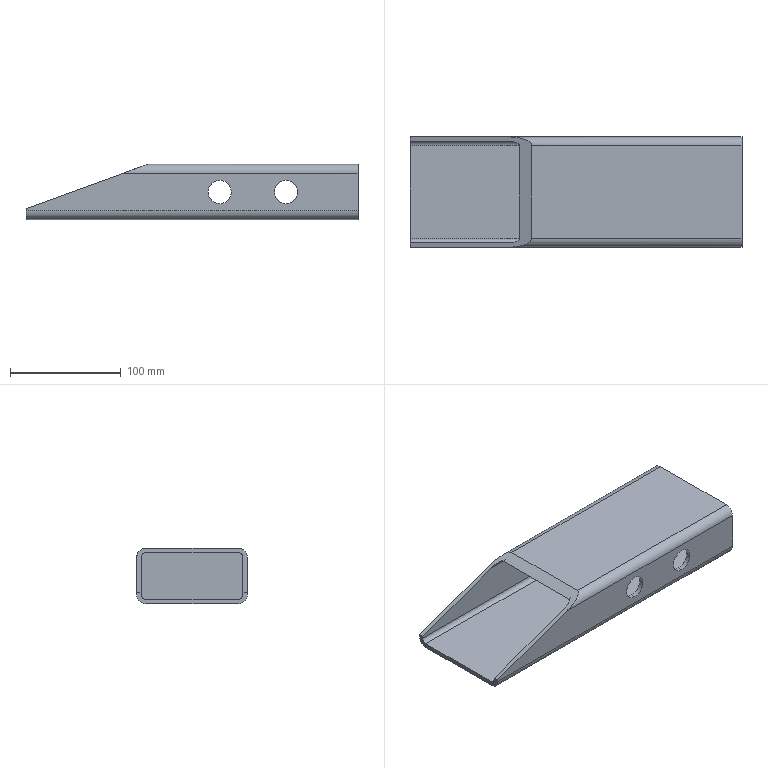Part | SolidWorks | features ICE 2, 3DProfileFeature 1, WeldMemberFeat 1, WeldmentFeature 1 | 2 solids | 37 faces | box 300 x 100 x 50 mm | volume 365371 mm3 | cylinder 20 | plane 17 | commonest cylinder face diameters 8 x8 21 x8 16 x4
STEP:
#1=CARTESIAN_POINT('',(235.,50.,-10.5));
#2=VERTEX_POINT('',#1);
#3=CARTESIAN_POINT('',(235.,50.,10.5));
#4=VERTEX_POINT('',#3);
#5=CARTESIAN_POINT('',(235.,50.,0.));
#6=DIRECTION('',(0.,1.,0.));
#7=DIRECTION('',(0.,0.,-1.));
#8=AXIS2_PLACEMENT_3D('',#5,#6,#7);
#9=CIRCLE('',#8,10.5);
#10=EDGE_CURVE('',#2,#4,#9,.T.);
#11=ORIENTED_EDGE('',*,*,#10,.T.);
#12=CARTESIAN_POINT('',(235.,46.,10.5));
#13=VERTEX_POINT('',#12);
#14=CARTESIAN_POINT('',(235.,166.952,10.5));
#15=DIRECTION('',(0.,-1.,0.));
#16=VECTOR('',#15,1000.);
#17=LINE('',#14,#16);
#18=EDGE_CURVE('',#4,#13,#17,.T.);
#19=ORIENTED_EDGE('',*,*,#18,.T.);
#20=CARTESIAN_POINT('',(235.,46.,-10.5));
#21=VERTEX_POINT('',#20);
#22=CARTESIAN_POINT('',(235.,46.,0.));
#23=DIRECTION('',(0.,-1.,0.));
#24=DIRECTION('',(0.,0.,-1.));
#25=AXIS2_PLACEMENT_3D('',#22,#23,#24);
#26=CIRCLE('',#25,10.5);
#27=EDGE_CURVE('',#13,#21,#26,.T.);
#28=ORIENTED_EDGE('',*,*,#27,.T.);
#29=CARTESIAN_POINT('',(235.,166.952,-10.5));
#30=DIRECTION('',(0.,-1.,0.));
#31=VECTOR('',#30,1000.);
#32=LINE('',#29,#31);
#33=EDGE_CURVE('',#2,#21,#32,.T.);
#34=ORIENTED_EDGE('',*,*,#33,.F.);
#35=EDGE_LOOP('',(#11,#19,#28,#34));
#36=FACE_OUTER_BOUND('',#35,.T.);
#37=CARTESIAN_POINT('',(235.,166.952,0.));
#38=DIRECTION('',(0.,-1.,0.));
#39=DIRECTION('',(0.,0.,-1.));
#40=AXIS2_PLACEMENT_3D('',#37,#38,#39);
#41=CYLINDRICAL_SURFACE('',#40,10.5);
#42=ADVANCED_FACE('',(#36),#41,.F.);
#43=CARTESIAN_POINT('',(175.,50.,-10.5));
#44=VERTEX_POINT('',#43);
#45=CARTESIAN_POINT('',(175.,50.,10.5));
#46=VERTEX_POINT('',#45);
#47=CARTESIAN_POINT('',(175.,50.,0.));
#48=DIRECTION('',(0.,1.,0.));
#49=DIRECTION('',(0.,0.,-1.));
#50=AXIS2_PLACEMENT_3D('',#47,#48,#49);
#51=CIRCLE('',#50,10.5);
#52=EDGE_CURVE('',#44,#46,#51,.T.);
#53=ORIENTED_EDGE('',*,*,#52,.T.);
#54=CARTESIAN_POINT('',(175.,46.,10.5));
#55=VERTEX_POINT('',#54);
#56=CARTESIAN_POINT('',(175.,166.952,10.5));
#57=DIRECTION('',(0.,-1.,0.));
#58=VECTOR('',#57,1000.);
#59=LINE('',#56,#58);
#60=EDGE_CURVE('',#46,#55,#59,.T.);
#61=ORIENTED_EDGE('',*,*,#60,.T.);
#62=CARTESIAN_POINT('',(175.,46.,-10.5));
#63=VERTEX_POINT('',#62);
#64=CARTESIAN_POINT('',(175.,46.,0.));
#65=DIRECTION('',(0.,-1.,0.));
#66=DIRECTION('',(0.,0.,-1.));
#67=AXIS2_PLACEMENT_3D('',#64,#65,#66);
#68=CIRCLE('',#67,10.5);
#69=EDGE_CURVE('',#55,#63,#68,.T.);
#70=ORIENTED_EDGE('',*,*,#69,.T.);
#71=CARTESIAN_POINT('',(175.,166.952,-10.5));
#72=DIRECTION('',(0.,-1.,0.));
#73=VECTOR('',#72,1000.);
#74=LINE('',#71,#73);
#75=EDGE_CURVE('',#44,#63,#74,.T.);
#76=ORIENTED_EDGE('',*,*,#75,.F.);
#77=EDGE_LOOP('',(#53,#61,#70,#76));
#78=FACE_OUTER_BOUND('',#77,.T.);
#79=CARTESIAN_POINT('',(175.,166.952,0.));
#80=DIRECTION('',(0.,-1.,0.));
#81=DIRECTION('',(0.,0.,-1.));
#82=AXIS2_PLACEMENT_3D('',#79,#80,#81);
#83=CYLINDRICAL_SURFACE('',#82,10.5);
#84=ADVANCED_FACE('',(#78),#83,.F.);
#85=CARTESIAN_POINT('',(235.,-46.,-10.5));
#86=VERTEX_POINT('',#85);
#87=CARTESIAN_POINT('',(235.,-46.,10.5));
#88=VERTEX_POINT('',#87);
#89=CARTESIAN_POINT('',(235.,-46.,0.));
#90=DIRECTION('',(0.,1.,0.));
#91=DIRECTION('',(0.,0.,1.));
#92=AXIS2_PLACEMENT_3D('',#89,#90,#91);
#93=CIRCLE('',#92,10.5);
#94=EDGE_CURVE('',#86,#88,#93,.T.);
#95=ORIENTED_EDGE('',*,*,#94,.T.);
#96=CARTESIAN_POINT('',(235.,-50.,10.5));
#97=VERTEX_POINT('',#96);
#98=CARTESIAN_POINT('',(235.,166.952,10.5));
#99=DIRECTION('',(0.,-1.,0.));
#100=VECTOR('',#99,1000.);
#101=LINE('',#98,#100);
#102=EDGE_CURVE('',#88,#97,#101,.T.);
#103=ORIENTED_EDGE('',*,*,#102,.T.);
#104=CARTESIAN_POINT('',(235.,-50.,-10.5));
#105=VERTEX_POINT('',#104);
#106=CARTESIAN_POINT('',(235.,-50.,0.));
#107=DIRECTION('',(0.,-1.,0.));
#108=DIRECTION('',(0.,0.,-1.));
#109=AXIS2_PLACEMENT_3D('',#106,#107,#108);
#110=CIRCLE('',#109,10.5);
#111=EDGE_CURVE('',#97,#105,#110,.T.);
#112=ORIENTED_EDGE('',*,*,#111,.T.);
#113=CARTESIAN_POINT('',(235.,166.952,-10.5));
#114=DIRECTION('',(0.,-1.,0.));
#115=VECTOR('',#114,1000.);
#116=LINE('',#113,#115);
#117=EDGE_CURVE('',#86,#105,#116,.T.);
#118=ORIENTED_EDGE('',*,*,#117,.F.);
#119=EDGE_LOOP('',(#95,#103,#112,#118));
#120=FACE_OUTER_BOUND('',#119,.T.);
#121=CARTESIAN_POINT('',(235.,166.952,0.));
#122=DIRECTION('',(0.,-1.,0.));
#123=DIRECTION('',(0.,0.,-1.));
#124=AXIS2_PLACEMENT_3D('',#121,#122,#123);
#125=CYLINDRICAL_SURFACE('',#124,10.5);
#126=ADVANCED_FACE('',(#120),#125,.F.);
#127=CARTESIAN_POINT('',(175.,-46.,-10.5));
#128=VERTEX_POINT('',#127);
#129=CARTESIAN_POINT('',(175.,-46.,10.5));
#130=VERTEX_POINT('',#129);
#131=CARTESIAN_POINT('',(175.,-46.,0.));
#132=DIRECTION('',(0.,1.,0.));
#133=DIRECTION('',(0.,0.,1.));
#134=AXIS2_PLACEMENT_3D('',#131,#132,#133);
#135=CIRCLE('',#134,10.5);
#136=EDGE_CURVE('',#128,#130,#135,.T.);
#137=ORIENTED_EDGE('',*,*,#136,.T.);
#138=CARTESIAN_POINT('',(175.,-50.,10.5));
#139=VERTEX_POINT('',#138);
#140=CARTESIAN_POINT('',(175.,166.952,10.5));
#141=DIRECTION('',(0.,-1.,0.));
#142=VECTOR('',#141,1000.);
#143=LINE('',#140,#142);
#144=EDGE_CURVE('',#130,#139,#143,.T.);
#145=ORIENTED_EDGE('',*,*,#144,.T.);
#146=CARTESIAN_POINT('',(175.,-50.,-10.5));
#147=VERTEX_POINT('',#146);
#148=CARTESIAN_POINT('',(175.,-50.,0.));
#149=DIRECTION('',(0.,-1.,0.));
#150=DIRECTION('',(0.,0.,-1.));
#151=AXIS2_PLACEMENT_3D('',#148,#149,#150);
#152=CIRCLE('',#151,10.5);
#153=EDGE_CURVE('',#139,#147,#152,.T.);
#154=ORIENTED_EDGE('',*,*,#153,.T.);
#155=CARTESIAN_POINT('',(175.,166.952,-10.5));
#156=DIRECTION('',(0.,-1.,0.));
#157=VECTOR('',#156,1000.);
#158=LINE('',#155,#157);
#159=EDGE_CURVE('',#128,#147,#158,.T.);
#160=ORIENTED_EDGE('',*,*,#159,.F.);
#161=EDGE_LOOP('',(#137,#145,#154,#160));
#162=FACE_OUTER_BOUND('',#161,.T.);
#163=CARTESIAN_POINT('',(175.,166.952,0.));
#164=DIRECTION('',(0.,-1.,0.));
#165=DIRECTION('',(0.,0.,-1.));
#166=AXIS2_PLACEMENT_3D('',#163,#164,#165);
#167=CYLINDRICAL_SURFACE('',#166,10.5);
#168=ADVANCED_FACE('',(#162),#167,.F.);
#169=CARTESIAN_POINT('',(0.,42.,-25.));
#170=VERTEX_POINT('',#169);
#171=CARTESIAN_POINT('',(0.,50.,-17.));
#172=VERTEX_POINT('',#171);
#173=CARTESIAN_POINT('',(0.,42.,-17.));
#174=DIRECTION('',(1.,0.,0.));
#175=DIRECTION('',(0.,0.,-1.));
#176=AXIS2_PLACEMENT_3D('',#173,#174,#175);
#177=CIRCLE('',#176,8.);
#178=EDGE_CURVE('',#170,#172,#177,.T.);
#179=ORIENTED_EDGE('',*,*,#178,.T.);
#180=CARTESIAN_POINT('',(300.,50.,-17.));
#181=VERTEX_POINT('',#180);
#182=CARTESIAN_POINT('',(300.,50.,-17.));
#183=DIRECTION('',(-1.,0.,0.));
#184=VECTOR('',#183,1000.);
#185=LINE('',#182,#184);
#186=EDGE_CURVE('',#181,#172,#185,.T.);
#187=ORIENTED_EDGE('',*,*,#186,.F.);
#188=CARTESIAN_POINT('',(300.,42.,-25.));
#189=VERTEX_POINT('',#188);
#190=CARTESIAN_POINT('',(300.,42.,-17.));
#191=DIRECTION('',(1.,0.,0.));
#192=DIRECTION('',(0.,0.,-1.));
#193=AXIS2_PLACEMENT_3D('',#190,#191,#192);
#194=CIRCLE('',#193,8.);
#195=EDGE_CURVE('',#189,#181,#194,.T.);
#196=ORIENTED_EDGE('',*,*,#195,.F.);
#197=CARTESIAN_POINT('',(300.,42.,-25.));
#198=DIRECTION('',(-1.,0.,0.));
#199=VECTOR('',#198,1000.);
#200=LINE('',#197,#199);
#201=EDGE_CURVE('',#189,#170,#200,.T.);
#202=ORIENTED_EDGE('',*,*,#201,.T.);
#203=EDGE_LOOP('',(#179,#187,#196,#202));
#204=FACE_OUTER_BOUND('',#203,.T.);
#205=CARTESIAN_POINT('',(300.,42.,-17.));
#206=DIRECTION('',(-1.,0.,0.));
#207=DIRECTION('',(0.,0.,1.));
#208=AXIS2_PLACEMENT_3D('',#205,#206,#207);
#209=CYLINDRICAL_SURFACE('',#208,8.);
#210=ADVANCED_FACE('',(#204),#209,.T.);
#211=ORIENTED_EDGE('',*,*,#10,.F.);
#212=CARTESIAN_POINT('',(235.,50.,0.));
#213=DIRECTION('',(0.,1.,0.));
#214=DIRECTION('',(0.,0.,-1.));
#215=AXIS2_PLACEMENT_3D('',#212,#213,#214);
#216=CIRCLE('',#215,10.5);
#217=EDGE_CURVE('',#4,#2,#216,.T.);
#218=ORIENTED_EDGE('',*,*,#217,.F.);
#219=EDGE_LOOP('',(#211,#218));
#220=FACE_BOUND('',#219,.T.);
#221=ORIENTED_EDGE('',*,*,#52,.F.);
#222=CARTESIAN_POINT('',(175.,50.,0.));
#223=DIRECTION('',(0.,1.,0.));
#224=DIRECTION('',(0.,0.,-1.));
#225=AXIS2_PLACEMENT_3D('',#222,#223,#224);
#226=CIRCLE('',#225,10.5);
#227=EDGE_CURVE('',#46,#44,#226,.T.);
#228=ORIENTED_EDGE('',*,*,#227,.F.);
#229=EDGE_LOOP('',(#221,#228));
#230=FACE_BOUND('',#229,.T.);
#231=CARTESIAN_POINT('',(0.,50.,-15.));
#232=VERTEX_POINT('',#231);
#233=CARTESIAN_POINT('',(0.,50.,-17.));
#234=DIRECTION('',(0.,0.,1.));
#235=VECTOR('',#234,1000.);
#236=LINE('',#233,#235);
#237=EDGE_CURVE('',#172,#232,#236,.T.);
#238=ORIENTED_EDGE('',*,*,#237,.T.);
#239=CARTESIAN_POINT('',(87.919,50.,17.));
#240=VERTEX_POINT('',#239);
#241=CARTESIAN_POINT('',(0.,50.,-15.));
#242=DIRECTION('',(-0.9397,0.,-0.342));
#243=VECTOR('',#242,1000.);
#244=LINE('',#241,#243);
#245=EDGE_CURVE('',#240,#232,#244,.T.);
#246=ORIENTED_EDGE('',*,*,#245,.F.);
#247=CARTESIAN_POINT('',(300.,50.,17.));
#248=VERTEX_POINT('',#247);
#249=CARTESIAN_POINT('',(300.,50.,17.));
#250=DIRECTION('',(-1.,0.,0.));
#251=VECTOR('',#250,1000.);
#252=LINE('',#249,#251);
#253=EDGE_CURVE('',#248,#240,#252,.T.);
#254=ORIENTED_EDGE('',*,*,#253,.F.);
#255=CARTESIAN_POINT('',(300.,50.,-17.));
#256=DIRECTION('',(0.,0.,1.));
#257=VECTOR('',#256,1000.);
#258=LINE('',#255,#257);
#259=EDGE_CURVE('',#181,#248,#258,.T.);
#260=ORIENTED_EDGE('',*,*,#259,.F.);
#261=ORIENTED_EDGE('',*,*,#186,.T.);
#262=EDGE_LOOP('',(#238,#246,#254,#260,#261));
#263=FACE_OUTER_BOUND('',#262,.T.);
#264=CARTESIAN_POINT('',(300.,50.,-17.));
#265=DIRECTION('',(0.,-1.,0.));
#266=DIRECTION('',(0.,0.,-1.));
#267=AXIS2_PLACEMENT_3D('',#264,#265,#266);
#268=PLANE('',#267);
#269=ADVANCED_FACE('',(#220,#230,#263),#268,.F.);
#270=ORIENTED_EDGE('',*,*,#253,.T.);
#271=CARTESIAN_POINT('',(109.899,42.,25.));
#272=VERTEX_POINT('',#271);
#273=CARTESIAN_POINT('',(87.919,50.,17.));
#274=CARTESIAN_POINT('',(100.795,50.,21.686));
#275=CARTESIAN_POINT('',(109.899,46.686,25.));
#276=CARTESIAN_POINT('',(109.899,42.,25.));
#277=(BOUNDED_CURVE()B_SPLINE_CURVE(3,(#273,#274,#275,#276),.UNSPECIFIED.,.F.,.F.)B_SPLINE_CURVE_WITH_KNOTS((4,4),(1.571,3.142),.UNSPECIFIED.)CURVE()GEOMETRIC_REPRESENTATION_ITEM()RATIONAL_B_SPLINE_CURVE((1.,0.8047,0.8047,1.))REPRESENTATION_ITEM(''));
#278=EDGE_CURVE('',#240,#272,#277,.T.);
#279=ORIENTED_EDGE('',*,*,#278,.T.);
#280=CARTESIAN_POINT('',(300.,42.,25.));
#281=VERTEX_POINT('',#280);
#282=CARTESIAN_POINT('',(300.,42.,25.));
#283=DIRECTION('',(-1.,0.,0.));
#284=VECTOR('',#283,1000.);
#285=LINE('',#282,#284);
#286=EDGE_CURVE('',#281,#272,#285,.T.);
#287=ORIENTED_EDGE('',*,*,#286,.F.);
#288=CARTESIAN_POINT('',(300.,42.,17.));
#289=DIRECTION('',(1.,0.,0.));
#290=DIRECTION('',(0.,0.,-1.));
#291=AXIS2_PLACEMENT_3D('',#288,#289,#290);
#292=CIRCLE('',#291,8.);
#293=EDGE_CURVE('',#248,#281,#292,.T.);
#294=ORIENTED_EDGE('',*,*,#293,.F.);
#295=EDGE_LOOP('',(#270,#279,#287,#294));
#296=FACE_OUTER_BOUND('',#295,.T.);
#297=CARTESIAN_POINT('',(300.,42.,17.));
#298=DIRECTION('',(-1.,0.,0.));
#299=DIRECTION('',(0.,0.,1.));
#300=AXIS2_PLACEMENT_3D('',#297,#298,#299);
#301=CYLINDRICAL_SURFACE('',#300,8.);
#302=ADVANCED_FACE('',(#296),#301,.T.);
#303=ORIENTED_EDGE('',*,*,#286,.T.);
#304=CARTESIAN_POINT('',(109.899,-42.,25.));
#305=VERTEX_POINT('',#304);
#306=CARTESIAN_POINT('',(109.899,166.952,25.));
#307=DIRECTION('',(0.,-1.,0.));
#308=VECTOR('',#307,1000.);
#309=LINE('',#306,#308);
#310=EDGE_CURVE('',#272,#305,#309,.T.);
#311=ORIENTED_EDGE('',*,*,#310,.T.);
#312=CARTESIAN_POINT('',(300.,-42.,25.));
#313=VERTEX_POINT('',#312);
#314=CARTESIAN_POINT('',(300.,-42.,25.));
#315=DIRECTION('',(-1.,0.,0.));
#316=VECTOR('',#315,1000.);
#317=LINE('',#314,#316);
#318=EDGE_CURVE('',#313,#305,#317,.T.);
#319=ORIENTED_EDGE('',*,*,#318,.F.);
#320=CARTESIAN_POINT('',(300.,-42.,25.));
#321=DIRECTION('',(0.,-1.,0.));
#322=VECTOR('',#321,1000.);
#323=LINE('',#320,#322);
#324=EDGE_CURVE('',#281,#313,#323,.T.);
#325=ORIENTED_EDGE('',*,*,#324,.F.);
#326=EDGE_LOOP('',(#303,#311,#319,#325));
#327=FACE_OUTER_BOUND('',#326,.T.);
#328=CARTESIAN_POINT('',(300.,-42.,25.));
#329=DIRECTION('',(0.,0.,-1.));
#330=DIRECTION('',(-1.,0.,0.));
#331=AXIS2_PLACEMENT_3D('',#328,#329,#330);
#332=PLANE('',#331);
#333=ADVANCED_FACE('',(#327),#332,.F.);
#334=ORIENTED_EDGE('',*,*,#318,.T.);
#335=CARTESIAN_POINT('',(87.919,-50.,17.));
#336=VERTEX_POINT('',#335);
#337=CARTESIAN_POINT('',(109.899,-42.,25.));
#338=CARTESIAN_POINT('',(109.899,-46.686,25.));
#339=CARTESIAN_POINT('',(100.795,-50.,21.686));
#340=CARTESIAN_POINT('',(87.919,-50.,17.));
#341=(BOUNDED_CURVE()B_SPLINE_CURVE(3,(#337,#338,#339,#340),.UNSPECIFIED.,.F.,.F.)B_SPLINE_CURVE_WITH_KNOTS((4,4),(3.142,4.712),.UNSPECIFIED.)CURVE()GEOMETRIC_REPRESENTATION_ITEM()RATIONAL_B_SPLINE_CURVE((1.,0.8047,0.8047,1.))REPRESENTATION_ITEM(''));
#342=EDGE_CURVE('',#305,#336,#341,.T.);
#343=ORIENTED_EDGE('',*,*,#342,.T.);
#344=CARTESIAN_POINT('',(300.,-50.,17.));
#345=VERTEX_POINT('',#344);
#346=CARTESIAN_POINT('',(300.,-50.,17.));
#347=DIRECTION('',(-1.,0.,0.));
#348=VECTOR('',#347,1000.);
#349=LINE('',#346,#348);
#350=EDGE_CURVE('',#345,#336,#349,.T.);
#351=ORIENTED_EDGE('',*,*,#350,.F.);
#352=CARTESIAN_POINT('',(300.,-42.,17.));
#353=DIRECTION('',(1.,0.,0.));
#354=DIRECTION('',(0.,0.,-1.));
#355=AXIS2_PLACEMENT_3D('',#352,#353,#354);
#356=CIRCLE('',#355,8.);
#357=EDGE_CURVE('',#313,#345,#356,.T.);
#358=ORIENTED_EDGE('',*,*,#357,.F.);
#359=EDGE_LOOP('',(#334,#343,#351,#358));
#360=FACE_OUTER_BOUND('',#359,.T.);
#361=CARTESIAN_POINT('',(300.,-42.,17.));
#362=DIRECTION('',(-1.,0.,0.));
#363=DIRECTION('',(0.,0.,1.));
#364=AXIS2_PLACEMENT_3D('',#361,#362,#363);
#365=CYLINDRICAL_SURFACE('',#364,8.);
#366=ADVANCED_FACE('',(#360),#365,.T.);
#367=CARTESIAN_POINT('',(235.,-50.,0.));
#368=DIRECTION('',(0.,-1.,0.));
#369=DIRECTION('',(0.,0.,-1.));
#370=AXIS2_PLACEMENT_3D('',#367,#368,#369);
#371=CIRCLE('',#370,10.5);
#372=EDGE_CURVE('',#105,#97,#371,.T.);
#373=ORIENTED_EDGE('',*,*,#372,.F.);
#374=ORIENTED_EDGE('',*,*,#111,.F.);
#375=EDGE_LOOP('',(#373,#374));
#376=FACE_BOUND('',#375,.T.);
#377=CARTESIAN_POINT('',(175.,-50.,0.));
#378=DIRECTION('',(0.,-1.,0.));
#379=DIRECTION('',(0.,0.,-1.));
#380=AXIS2_PLACEMENT_3D('',#377,#378,#379);
#381=CIRCLE('',#380,10.5);
#382=EDGE_CURVE('',#147,#139,#381,.T.);
#383=ORIENTED_EDGE('',*,*,#382,.F.);
#384=ORIENTED_EDGE('',*,*,#153,.F.);
#385=EDGE_LOOP('',(#383,#384));
#386=FACE_BOUND('',#385,.T.);
#387=ORIENTED_EDGE('',*,*,#350,.T.);
#388=CARTESIAN_POINT('',(0.,-50.,-15.));
#389=VERTEX_POINT('',#388);
#390=CARTESIAN_POINT('',(0.,-50.,-15.));
#391=DIRECTION('',(0.9397,0.,0.342));
#392=VECTOR('',#391,1000.);
#393=LINE('',#390,#392);
#394=EDGE_CURVE('',#389,#336,#393,.T.);
#395=ORIENTED_EDGE('',*,*,#394,.F.);
#396=CARTESIAN_POINT('',(0.,-50.,-17.));
#397=VERTEX_POINT('',#396);
#398=CARTESIAN_POINT('',(0.,-50.,17.));
#399=DIRECTION('',(0.,0.,-1.));
#400=VECTOR('',#399,1000.);
#401=LINE('',#398,#400);
#402=EDGE_CURVE('',#389,#397,#401,.T.);
#403=ORIENTED_EDGE('',*,*,#402,.T.);
#404=CARTESIAN_POINT('',(300.,-50.,-17.));
#405=VERTEX_POINT('',#404);
#406=CARTESIAN_POINT('',(300.,-50.,-17.));
#407=DIRECTION('',(-1.,0.,0.));
#408=VECTOR('',#407,1000.);
#409=LINE('',#406,#408);
#410=EDGE_CURVE('',#405,#397,#409,.T.);
#411=ORIENTED_EDGE('',*,*,#410,.F.);
#412=CARTESIAN_POINT('',(300.,-50.,17.));
#413=DIRECTION('',(0.,0.,-1.));
#414=VECTOR('',#413,1000.);
#415=LINE('',#412,#414);
#416=EDGE_CURVE('',#345,#405,#415,.T.);
#417=ORIENTED_EDGE('',*,*,#416,.F.);
#418=EDGE_LOOP('',(#387,#395,#403,#411,#417));
#419=FACE_OUTER_BOUND('',#418,.T.);
#420=CARTESIAN_POINT('',(300.,-50.,17.));
#421=DIRECTION('',(0.,1.,0.));
#422=DIRECTION('',(0.,0.,1.));
#423=AXIS2_PLACEMENT_3D('',#420,#421,#422);
#424=PLANE('',#423);
#425=ADVANCED_FACE('',(#376,#386,#419),#424,.F.);
#426=CARTESIAN_POINT('',(0.,-42.,-25.));
#427=VERTEX_POINT('',#426);
#428=CARTESIAN_POINT('',(0.,-42.,-17.));
#429=DIRECTION('',(1.,0.,0.));
#430=DIRECTION('',(0.,0.,-1.));
#431=AXIS2_PLACEMENT_3D('',#428,#429,#430);
#432=CIRCLE('',#431,8.);
#433=EDGE_CURVE('',#397,#427,#432,.T.);
#434=ORIENTED_EDGE('',*,*,#433,.T.);
#435=CARTESIAN_POINT('',(300.,-42.,-25.));
#436=VERTEX_POINT('',#435);
#437=CARTESIAN_POINT('',(300.,-42.,-25.));
#438=DIRECTION('',(-1.,0.,0.));
#439=VECTOR('',#438,1000.);
#440=LINE('',#437,#439);
#441=EDGE_CURVE('',#436,#427,#440,.T.);
#442=ORIENTED_EDGE('',*,*,#441,.F.);
#443=CARTESIAN_POINT('',(300.,-42.,-17.));
#444=DIRECTION('',(1.,0.,0.));
#445=DIRECTION('',(0.,0.,-1.));
#446=AXIS2_PLACEMENT_3D('',#443,#444,#445);
#447=CIRCLE('',#446,8.);
#448=EDGE_CURVE('',#405,#436,#447,.T.);
#449=ORIENTED_EDGE('',*,*,#448,.F.);
#450=ORIENTED_EDGE('',*,*,#410,.T.);
#451=EDGE_LOOP('',(#434,#442,#449,#450));
#452=FACE_OUTER_BOUND('',#451,.T.);
#453=CARTESIAN_POINT('',(300.,-42.,-17.));
#454=DIRECTION('',(-1.,0.,0.));
#455=DIRECTION('',(0.,0.,1.));
#456=AXIS2_PLACEMENT_3D('',#453,#454,#455);
#457=CYLINDRICAL_SURFACE('',#456,8.);
#458=ADVANCED_FACE('',(#452),#457,.T.);
#459=CARTESIAN_POINT('',(87.919,46.,17.));
#460=VERTEX_POINT('',#459);
#461=CARTESIAN_POINT('',(98.909,42.,21.));
#462=VERTEX_POINT('',#461);
#463=CARTESIAN_POINT('',(87.919,46.,17.));
#464=CARTESIAN_POINT('',(94.357,46.,19.343));
#465=CARTESIAN_POINT('',(98.909,44.343,21.));
#466=CARTESIAN_POINT('',(98.909,42.,21.));
#467=(BOUNDED_CURVE()B_SPLINE_CURVE(3,(#463,#464,#465,#466),.UNSPECIFIED.,.F.,.F.)B_SPLINE_CURVE_WITH_KNOTS((4,4),(1.571,3.142),.UNSPECIFIED.)CURVE()GEOMETRIC_REPRESENTATION_ITEM()RATIONAL_B_SPLINE_CURVE((1.,0.8047,0.8047,1.))REPRESENTATION_ITEM(''));
#468=EDGE_CURVE('',#460,#462,#467,.T.);
#469=ORIENTED_EDGE('',*,*,#468,.F.);
#470=CARTESIAN_POINT('',(300.,46.,17.));
#471=VERTEX_POINT('',#470);
#472=CARTESIAN_POINT('',(300.,46.,17.));
#473=DIRECTION('',(-1.,0.,0.));
#474=VECTOR('',#473,1000.);
#475=LINE('',#472,#474);
#476=EDGE_CURVE('',#471,#460,#475,.T.);
#477=ORIENTED_EDGE('',*,*,#476,.F.);
#478=CARTESIAN_POINT('',(300.,42.,21.));
#479=VERTEX_POINT('',#478);
#480=CARTESIAN_POINT('',(300.,42.,17.));
#481=DIRECTION('',(1.,0.,0.));
#482=DIRECTION('',(0.,0.,-1.));
#483=AXIS2_PLACEMENT_3D('',#480,#481,#482);
#484=CIRCLE('',#483,4.);
#485=EDGE_CURVE('',#471,#479,#484,.T.);
#486=ORIENTED_EDGE('',*,*,#485,.T.);
#487=CARTESIAN_POINT('',(300.,42.,21.));
#488=DIRECTION('',(-1.,0.,0.));
#489=VECTOR('',#488,1000.);
#490=LINE('',#487,#489);
#491=EDGE_CURVE('',#479,#462,#490,.T.);
#492=ORIENTED_EDGE('',*,*,#491,.T.);
#493=EDGE_LOOP('',(#469,#477,#486,#492));
#494=FACE_OUTER_BOUND('',#493,.T.);
#495=CARTESIAN_POINT('',(300.,42.,17.));
#496=DIRECTION('',(-1.,0.,0.));
#497=DIRECTION('',(0.,0.,1.));
#498=AXIS2_PLACEMENT_3D('',#495,#496,#497);
#499=CYLINDRICAL_SURFACE('',#498,4.);
#500=ADVANCED_FACE('',(#494),#499,.F.);
#501=CARTESIAN_POINT('',(235.,46.,0.));
#502=DIRECTION('',(0.,-1.,0.));
#503=DIRECTION('',(0.,0.,-1.));
#504=AXIS2_PLACEMENT_3D('',#501,#502,#503);
#505=CIRCLE('',#504,10.5);
#506=EDGE_CURVE('',#21,#13,#505,.T.);
#507=ORIENTED_EDGE('',*,*,#506,.F.);
#508=ORIENTED_EDGE('',*,*,#27,.F.);
#509=EDGE_LOOP('',(#507,#508));
#510=FACE_BOUND('',#509,.T.);
#511=CARTESIAN_POINT('',(175.,46.,0.));
#512=DIRECTION('',(0.,-1.,0.));
#513=DIRECTION('',(0.,0.,-1.));
#514=AXIS2_PLACEMENT_3D('',#511,#512,#513);
#515=CIRCLE('',#514,10.5);
#516=EDGE_CURVE('',#63,#55,#515,.T.);
#517=ORIENTED_EDGE('',*,*,#516,.F.);
#518=ORIENTED_EDGE('',*,*,#69,.F.);
#519=EDGE_LOOP('',(#517,#518));
#520=FACE_BOUND('',#519,.T.);
#521=CARTESIAN_POINT('',(0.,46.,-15.));
#522=VERTEX_POINT('',#521);
#523=CARTESIAN_POINT('',(264.264,46.,81.184));
#524=DIRECTION('',(0.9397,0.,0.342));
#525=VECTOR('',#524,1000.);
#526=LINE('',#523,#525);
#527=EDGE_CURVE('',#522,#460,#526,.T.);
#528=ORIENTED_EDGE('',*,*,#527,.F.);
#529=CARTESIAN_POINT('',(0.,46.,-17.));
#530=VERTEX_POINT('',#529);
#531=CARTESIAN_POINT('',(0.,46.,-17.));
#532=DIRECTION('',(0.,0.,1.));
#533=VECTOR('',#532,1000.);
#534=LINE('',#531,#533);
#535=EDGE_CURVE('',#530,#522,#534,.T.);
#536=ORIENTED_EDGE('',*,*,#535,.F.);
#537=CARTESIAN_POINT('',(300.,46.,-17.));
#538=VERTEX_POINT('',#537);
#539=CARTESIAN_POINT('',(300.,46.,-17.));
#540=DIRECTION('',(-1.,0.,0.));
#541=VECTOR('',#540,1000.);
#542=LINE('',#539,#541);
#543=EDGE_CURVE('',#538,#530,#542,.T.);
#544=ORIENTED_EDGE('',*,*,#543,.F.);
#545=CARTESIAN_POINT('',(300.,46.,-17.));
#546=DIRECTION('',(0.,0.,1.));
#547=VECTOR('',#546,1000.);
#548=LINE('',#545,#547);
#549=EDGE_CURVE('',#538,#471,#548,.T.);
#550=ORIENTED_EDGE('',*,*,#549,.T.);
#551=ORIENTED_EDGE('',*,*,#476,.T.);
#552=EDGE_LOOP('',(#528,#536,#544,#550,#551));
#553=FACE_OUTER_BOUND('',#552,.T.);
#554=CARTESIAN_POINT('',(300.,46.,-17.));
#555=DIRECTION('',(0.,-1.,0.));
#556=DIRECTION('',(0.,0.,-1.));
#557=AXIS2_PLACEMENT_3D('',#554,#555,#556);
#558=PLANE('',#557);
#559=ADVANCED_FACE('',(#510,#520,#553),#558,.T.);
#560=CARTESIAN_POINT('',(0.,42.,-21.));
#561=VERTEX_POINT('',#560);
#562=CARTESIAN_POINT('',(0.,42.,-17.));
#563=DIRECTION('',(1.,0.,0.));
#564=DIRECTION('',(0.,0.,-1.));
#565=AXIS2_PLACEMENT_3D('',#562,#563,#564);
#566=CIRCLE('',#565,4.);
#567=EDGE_CURVE('',#561,#530,#566,.T.);
#568=ORIENTED_EDGE('',*,*,#567,.F.);
#569=CARTESIAN_POINT('',(300.,42.,-21.));
#570=VERTEX_POINT('',#569);
#571=CARTESIAN_POINT('',(300.,42.,-21.));
#572=DIRECTION('',(-1.,0.,0.));
#573=VECTOR('',#572,1000.);
#574=LINE('',#571,#573);
#575=EDGE_CURVE('',#570,#561,#574,.T.);
#576=ORIENTED_EDGE('',*,*,#575,.F.);
#577=CARTESIAN_POINT('',(300.,42.,-17.));
#578=DIRECTION('',(1.,0.,0.));
#579=DIRECTION('',(0.,0.,-1.));
#580=AXIS2_PLACEMENT_3D('',#577,#578,#579);
#581=CIRCLE('',#580,4.);
#582=EDGE_CURVE('',#570,#538,#581,.T.);
#583=ORIENTED_EDGE('',*,*,#582,.T.);
#584=ORIENTED_EDGE('',*,*,#543,.T.);
#585=EDGE_LOOP('',(#568,#576,#583,#584));
#586=FACE_OUTER_BOUND('',#585,.T.);
#587=CARTESIAN_POINT('',(300.,42.,-17.));
#588=DIRECTION('',(-1.,0.,0.));
#589=DIRECTION('',(0.,0.,1.));
#590=AXIS2_PLACEMENT_3D('',#587,#588,#589);
#591=CYLINDRICAL_SURFACE('',#590,4.);
#592=ADVANCED_FACE('',(#586),#591,.F.);
#593=CARTESIAN_POINT('',(0.,-42.,-21.));
#594=VERTEX_POINT('',#593);
#595=CARTESIAN_POINT('',(0.,42.,-21.));
#596=DIRECTION('',(0.,1.,0.));
#597=VECTOR('',#596,1000.);
#598=LINE('',#595,#597);
#599=EDGE_CURVE('',#594,#561,#598,.T.);
#600=ORIENTED_EDGE('',*,*,#599,.F.);
#601=CARTESIAN_POINT('',(300.,-42.,-21.));
#602=VERTEX_POINT('',#601);
#603=CARTESIAN_POINT('',(300.,-42.,-21.));
#604=DIRECTION('',(-1.,0.,0.));
#605=VECTOR('',#604,1000.);
#606=LINE('',#603,#605);
#607=EDGE_CURVE('',#602,#594,#606,.T.);
#608=ORIENTED_EDGE('',*,*,#607,.F.);
#609=CARTESIAN_POINT('',(300.,42.,-21.));
#610=DIRECTION('',(0.,1.,0.));
#611=VECTOR('',#610,1000.);
#612=LINE('',#609,#611);
#613=EDGE_CURVE('',#602,#570,#612,.T.);
#614=ORIENTED_EDGE('',*,*,#613,.T.);
#615=ORIENTED_EDGE('',*,*,#575,.T.);
#616=EDGE_LOOP('',(#600,#608,#614,#615));
#617=FACE_OUTER_BOUND('',#616,.T.);
#618=CARTESIAN_POINT('',(300.,42.,-21.));
#619=DIRECTION('',(0.,0.,1.));
#620=DIRECTION('',(1.,0.,0.));
#621=AXIS2_PLACEMENT_3D('',#618,#619,#620);
#622=PLANE('',#621);
#623=ADVANCED_FACE('',(#617),#622,.T.);
#624=CARTESIAN_POINT('',(0.,-46.,-17.));
#625=VERTEX_POINT('',#624);
#626=CARTESIAN_POINT('',(0.,-42.,-17.));
#627=DIRECTION('',(1.,0.,0.));
#628=DIRECTION('',(0.,0.,-1.));
#629=AXIS2_PLACEMENT_3D('',#626,#627,#628);
#630=CIRCLE('',#629,4.);
#631=EDGE_CURVE('',#625,#594,#630,.T.);
#632=ORIENTED_EDGE('',*,*,#631,.F.);
#633=CARTESIAN_POINT('',(300.,-46.,-17.));
#634=VERTEX_POINT('',#633);
#635=CARTESIAN_POINT('',(300.,-46.,-17.));
#636=DIRECTION('',(-1.,0.,0.));
#637=VECTOR('',#636,1000.);
#638=LINE('',#635,#637);
#639=EDGE_CURVE('',#634,#625,#638,.T.);
#640=ORIENTED_EDGE('',*,*,#639,.F.);
#641=CARTESIAN_POINT('',(300.,-42.,-17.));
#642=DIRECTION('',(1.,0.,0.));
#643=DIRECTION('',(0.,0.,-1.));
#644=AXIS2_PLACEMENT_3D('',#641,#642,#643);
#645=CIRCLE('',#644,4.);
#646=EDGE_CURVE('',#634,#602,#645,.T.);
#647=ORIENTED_EDGE('',*,*,#646,.T.);
#648=ORIENTED_EDGE('',*,*,#607,.T.);
#649=EDGE_LOOP('',(#632,#640,#647,#648));
#650=FACE_OUTER_BOUND('',#649,.T.);
#651=CARTESIAN_POINT('',(300.,-42.,-17.));
#652=DIRECTION('',(-1.,0.,0.));
#653=DIRECTION('',(0.,0.,1.));
#654=AXIS2_PLACEMENT_3D('',#651,#652,#653);
#655=CYLINDRICAL_SURFACE('',#654,4.);
#656=ADVANCED_FACE('',(#650),#655,.F.);
#657=ORIENTED_EDGE('',*,*,#94,.F.);
#658=CARTESIAN_POINT('',(235.,-46.,0.));
#659=DIRECTION('',(0.,1.,0.));
#660=DIRECTION('',(0.,0.,1.));
#661=AXIS2_PLACEMENT_3D('',#658,#659,#660);
#662=CIRCLE('',#661,10.5);
#663=EDGE_CURVE('',#88,#86,#662,.T.);
#664=ORIENTED_EDGE('',*,*,#663,.F.);
#665=EDGE_LOOP('',(#657,#664));
#666=FACE_BOUND('',#665,.T.);
#667=ORIENTED_EDGE('',*,*,#136,.F.);
#668=CARTESIAN_POINT('',(175.,-46.,0.));
#669=DIRECTION('',(0.,1.,0.));
#670=DIRECTION('',(0.,0.,1.));
#671=AXIS2_PLACEMENT_3D('',#668,#669,#670);
#672=CIRCLE('',#671,10.5);
#673=EDGE_CURVE('',#130,#128,#672,.T.);
#674=ORIENTED_EDGE('',*,*,#673,.F.);
#675=EDGE_LOOP('',(#667,#674));
#676=FACE_BOUND('',#675,.T.);
#677=CARTESIAN_POINT('',(87.919,-46.,17.));
#678=VERTEX_POINT('',#677);
#679=CARTESIAN_POINT('',(0.,-46.,-15.));
#680=VERTEX_POINT('',#679);
#681=CARTESIAN_POINT('',(275.191,-46.,85.161));
#682=DIRECTION('',(-0.9397,0.,-0.342));
#683=VECTOR('',#682,1000.);
#684=LINE('',#681,#683);
#685=EDGE_CURVE('',#678,#680,#684,.T.);
#686=ORIENTED_EDGE('',*,*,#685,.F.);
#687=CARTESIAN_POINT('',(300.,-46.,17.));
#688=VERTEX_POINT('',#687);
#689=CARTESIAN_POINT('',(300.,-46.,17.));
#690=DIRECTION('',(-1.,0.,0.));
#691=VECTOR('',#690,1000.);
#692=LINE('',#689,#691);
#693=EDGE_CURVE('',#688,#678,#692,.T.);
#694=ORIENTED_EDGE('',*,*,#693,.F.);
#695=CARTESIAN_POINT('',(300.,-46.,17.));
#696=DIRECTION('',(0.,0.,-1.));
#697=VECTOR('',#696,1000.);
#698=LINE('',#695,#697);
#699=EDGE_CURVE('',#688,#634,#698,.T.);
#700=ORIENTED_EDGE('',*,*,#699,.T.);
#701=ORIENTED_EDGE('',*,*,#639,.T.);
#702=CARTESIAN_POINT('',(0.,-46.,17.));
#703=DIRECTION('',(0.,0.,-1.));
#704=VECTOR('',#703,1000.);
#705=LINE('',#702,#704);
#706=EDGE_CURVE('',#680,#625,#705,.T.);
#707=ORIENTED_EDGE('',*,*,#706,.F.);
#708=EDGE_LOOP('',(#686,#694,#700,#701,#707));
#709=FACE_OUTER_BOUND('',#708,.T.);
#710=CARTESIAN_POINT('',(300.,-46.,17.));
#711=DIRECTION('',(0.,1.,0.));
#712=DIRECTION('',(0.,0.,1.));
#713=AXIS2_PLACEMENT_3D('',#710,#711,#712);
#714=PLANE('',#713);
#715=ADVANCED_FACE('',(#666,#676,#709),#714,.T.);
#716=CARTESIAN_POINT('',(98.909,-42.,21.));
#717=VERTEX_POINT('',#716);
#718=CARTESIAN_POINT('',(98.909,-42.,21.));
#719=CARTESIAN_POINT('',(98.909,-44.343,21.));
#720=CARTESIAN_POINT('',(94.357,-46.,19.343));
#721=CARTESIAN_POINT('',(87.919,-46.,17.));
#722=(BOUNDED_CURVE()B_SPLINE_CURVE(3,(#718,#719,#720,#721),.UNSPECIFIED.,.F.,.F.)B_SPLINE_CURVE_WITH_KNOTS((4,4),(3.142,4.712),.UNSPECIFIED.)CURVE()GEOMETRIC_REPRESENTATION_ITEM()RATIONAL_B_SPLINE_CURVE((1.,0.8047,0.8047,1.))REPRESENTATION_ITEM(''));
#723=EDGE_CURVE('',#717,#678,#722,.T.);
#724=ORIENTED_EDGE('',*,*,#723,.F.);
#725=CARTESIAN_POINT('',(300.,-42.,21.));
#726=VERTEX_POINT('',#725);
#727=CARTESIAN_POINT('',(300.,-42.,21.));
#728=DIRECTION('',(-1.,0.,0.));
#729=VECTOR('',#728,1000.);
#730=LINE('',#727,#729);
#731=EDGE_CURVE('',#726,#717,#730,.T.);
#732=ORIENTED_EDGE('',*,*,#731,.F.);
#733=CARTESIAN_POINT('',(300.,-42.,17.));
#734=DIRECTION('',(1.,0.,0.));
#735=DIRECTION('',(0.,0.,-1.));
#736=AXIS2_PLACEMENT_3D('',#733,#734,#735);
#737=CIRCLE('',#736,4.);
#738=EDGE_CURVE('',#726,#688,#737,.T.);
#739=ORIENTED_EDGE('',*,*,#738,.T.);
#740=ORIENTED_EDGE('',*,*,#693,.T.);
#741=EDGE_LOOP('',(#724,#732,#739,#740));
#742=FACE_OUTER_BOUND('',#741,.T.);
#743=CARTESIAN_POINT('',(300.,-42.,17.));
#744=DIRECTION('',(-1.,0.,0.));
#745=DIRECTION('',(0.,0.,1.));
#746=AXIS2_PLACEMENT_3D('',#743,#744,#745);
#747=CYLINDRICAL_SURFACE('',#746,4.);
#748=ADVANCED_FACE('',(#742),#747,.F.);
#749=CARTESIAN_POINT('',(98.909,-42.,21.));
#750=DIRECTION('',(0.,-1.,0.));
#751=VECTOR('',#750,1000.);
#752=LINE('',#749,#751);
#753=EDGE_CURVE('',#462,#717,#752,.T.);
#754=ORIENTED_EDGE('',*,*,#753,.F.);
#755=ORIENTED_EDGE('',*,*,#491,.F.);
#756=CARTESIAN_POINT('',(300.,-42.,21.));
#757=DIRECTION('',(0.,-1.,0.));
#758=VECTOR('',#757,1000.);
#759=LINE('',#756,#758);
#760=EDGE_CURVE('',#479,#726,#759,.T.);
#761=ORIENTED_EDGE('',*,*,#760,.T.);
#762=ORIENTED_EDGE('',*,*,#731,.T.);
#763=EDGE_LOOP('',(#754,#755,#761,#762));
#764=FACE_OUTER_BOUND('',#763,.T.);
#765=CARTESIAN_POINT('',(300.,-42.,21.));
#766=DIRECTION('',(0.,0.,-1.));
#767=DIRECTION('',(-1.,0.,0.));
#768=AXIS2_PLACEMENT_3D('',#765,#766,#767);
#769=PLANE('',#768);
#770=ADVANCED_FACE('',(#764),#769,.T.);
#771=CARTESIAN_POINT('',(0.,42.,-25.));
#772=DIRECTION('',(0.,1.,0.));
#773=VECTOR('',#772,1000.);
#774=LINE('',#771,#773);
#775=EDGE_CURVE('',#427,#170,#774,.T.);
#776=ORIENTED_EDGE('',*,*,#775,.T.);
#777=ORIENTED_EDGE('',*,*,#201,.F.);
#778=CARTESIAN_POINT('',(300.,42.,-25.));
#779=DIRECTION('',(0.,1.,0.));
#780=VECTOR('',#779,1000.);
#781=LINE('',#778,#780);
#782=EDGE_CURVE('',#436,#189,#781,.T.);
#783=ORIENTED_EDGE('',*,*,#782,.F.);
#784=ORIENTED_EDGE('',*,*,#441,.T.);
#785=EDGE_LOOP('',(#776,#777,#783,#784));
#786=FACE_OUTER_BOUND('',#785,.T.);
#787=CARTESIAN_POINT('',(300.,42.,-25.));
#788=DIRECTION('',(0.,0.,1.));
#789=DIRECTION('',(1.,0.,0.));
#790=AXIS2_PLACEMENT_3D('',#787,#788,#789);
#791=PLANE('',#790);
#792=ADVANCED_FACE('',(#786),#791,.F.);
#793=ORIENTED_EDGE('',*,*,#485,.F.);
#794=ORIENTED_EDGE('',*,*,#549,.F.);
#795=ORIENTED_EDGE('',*,*,#582,.F.);
#796=ORIENTED_EDGE('',*,*,#613,.F.);
#797=ORIENTED_EDGE('',*,*,#646,.F.);
#798=ORIENTED_EDGE('',*,*,#699,.F.);
#799=ORIENTED_EDGE('',*,*,#738,.F.);
#800=ORIENTED_EDGE('',*,*,#760,.F.);
#801=EDGE_LOOP('',(#793,#794,#795,#796,#797,#798,#799,#800));
#802=FACE_BOUND('',#801,.T.);
#803=ORIENTED_EDGE('',*,*,#195,.T.);
#804=ORIENTED_EDGE('',*,*,#259,.T.);
#805=ORIENTED_EDGE('',*,*,#293,.T.);
#806=ORIENTED_EDGE('',*,*,#324,.T.);
#807=ORIENTED_EDGE('',*,*,#357,.T.);
#808=ORIENTED_EDGE('',*,*,#416,.T.);
#809=ORIENTED_EDGE('',*,*,#448,.T.);
#810=ORIENTED_EDGE('',*,*,#782,.T.);
#811=EDGE_LOOP('',(#803,#804,#805,#806,#807,#808,#809,#810));
#812=FACE_OUTER_BOUND('',#811,.T.);
#813=CARTESIAN_POINT('',(300.,42.,-17.));
#814=DIRECTION('',(1.,0.,0.));
#815=DIRECTION('',(0.,0.,-1.));
#816=AXIS2_PLACEMENT_3D('',#813,#814,#815);
#817=PLANE('',#816);
#818=ADVANCED_FACE('',(#802,#812),#817,.T.);
#819=ORIENTED_EDGE('',*,*,#402,.F.);
#820=CARTESIAN_POINT('',(0.,42.,-15.));
#821=DIRECTION('',(0.,1.,0.));
#822=VECTOR('',#821,1000.);
#823=LINE('',#820,#822);
#824=EDGE_CURVE('',#389,#680,#823,.T.);
#825=ORIENTED_EDGE('',*,*,#824,.T.);
#826=ORIENTED_EDGE('',*,*,#706,.T.);
#827=ORIENTED_EDGE('',*,*,#631,.T.);
#828=ORIENTED_EDGE('',*,*,#599,.T.);
#829=ORIENTED_EDGE('',*,*,#567,.T.);
#830=ORIENTED_EDGE('',*,*,#535,.T.);
#831=CARTESIAN_POINT('',(0.,166.952,-15.));
#832=DIRECTION('',(0.,-1.,0.));
#833=VECTOR('',#832,1000.);
#834=LINE('',#831,#833);
#835=EDGE_CURVE('',#232,#522,#834,.T.);
#836=ORIENTED_EDGE('',*,*,#835,.F.);
#837=ORIENTED_EDGE('',*,*,#237,.F.);
#838=ORIENTED_EDGE('',*,*,#178,.F.);
#839=ORIENTED_EDGE('',*,*,#775,.F.);
#840=ORIENTED_EDGE('',*,*,#433,.F.);
#841=EDGE_LOOP('',(#819,#825,#826,#827,#828,#829,#830,#836,#837,#838,#839,#840));
#842=FACE_OUTER_BOUND('',#841,.T.);
#843=CARTESIAN_POINT('',(0.,42.,-17.));
#844=DIRECTION('',(1.,0.,0.));
#845=DIRECTION('',(0.,0.,-1.));
#846=AXIS2_PLACEMENT_3D('',#843,#844,#845);
#847=PLANE('',#846);
#848=ADVANCED_FACE('',(#842),#847,.F.);
#849=ORIENTED_EDGE('',*,*,#245,.T.);
#850=ORIENTED_EDGE('',*,*,#835,.T.);
#851=ORIENTED_EDGE('',*,*,#527,.T.);
#852=ORIENTED_EDGE('',*,*,#468,.T.);
#853=ORIENTED_EDGE('',*,*,#753,.T.);
#854=ORIENTED_EDGE('',*,*,#723,.T.);
#855=ORIENTED_EDGE('',*,*,#685,.T.);
#856=ORIENTED_EDGE('',*,*,#824,.F.);
#857=ORIENTED_EDGE('',*,*,#394,.T.);
#858=ORIENTED_EDGE('',*,*,#342,.F.);
#859=ORIENTED_EDGE('',*,*,#310,.F.);
#860=ORIENTED_EDGE('',*,*,#278,.F.);
#861=EDGE_LOOP('',(#849,#850,#851,#852,#853,#854,#855,#856,#857,#858,#859,#860));
#862=FACE_OUTER_BOUND('',#861,.T.);
#863=CARTESIAN_POINT('',(0.,166.952,-15.));
#864=DIRECTION('',(0.342,0.,-0.9397));
#865=DIRECTION('',(-0.9397,0.,-0.342));
#866=AXIS2_PLACEMENT_3D('',#863,#864,#865);
#867=PLANE('',#866);
#868=ADVANCED_FACE('',(#862),#867,.F.);
#869=ORIENTED_EDGE('',*,*,#144,.F.);
#870=ORIENTED_EDGE('',*,*,#673,.T.);
#871=ORIENTED_EDGE('',*,*,#159,.T.);
#872=ORIENTED_EDGE('',*,*,#382,.T.);
#873=EDGE_LOOP('',(#869,#870,#871,#872));
#874=FACE_OUTER_BOUND('',#873,.T.);
#875=CARTESIAN_POINT('',(175.,166.952,0.));
#876=DIRECTION('',(0.,-1.,0.));
#877=DIRECTION('',(0.,0.,-1.));
#878=AXIS2_PLACEMENT_3D('',#875,#876,#877);
#879=CYLINDRICAL_SURFACE('',#878,10.5);
#880=ADVANCED_FACE('',(#874),#879,.F.);
#881=ORIENTED_EDGE('',*,*,#102,.F.);
#882=ORIENTED_EDGE('',*,*,#663,.T.);
#883=ORIENTED_EDGE('',*,*,#117,.T.);
#884=ORIENTED_EDGE('',*,*,#372,.T.);
#885=EDGE_LOOP('',(#881,#882,#883,#884));
#886=FACE_OUTER_BOUND('',#885,.T.);
#887=CARTESIAN_POINT('',(235.,166.952,0.));
#888=DIRECTION('',(0.,-1.,0.));
#889=DIRECTION('',(0.,0.,-1.));
#890=AXIS2_PLACEMENT_3D('',#887,#888,#889);
#891=CYLINDRICAL_SURFACE('',#890,10.5);
#892=ADVANCED_FACE('',(#886),#891,.F.);
#893=ORIENTED_EDGE('',*,*,#60,.F.);
#894=ORIENTED_EDGE('',*,*,#227,.T.);
#895=ORIENTED_EDGE('',*,*,#75,.T.);
#896=ORIENTED_EDGE('',*,*,#516,.T.);
#897=EDGE_LOOP('',(#893,#894,#895,#896));
#898=FACE_OUTER_BOUND('',#897,.T.);
#899=CARTESIAN_POINT('',(175.,166.952,0.));
#900=DIRECTION('',(0.,-1.,0.));
#901=DIRECTION('',(0.,0.,-1.));
#902=AXIS2_PLACEMENT_3D('',#899,#900,#901);
#903=CYLINDRICAL_SURFACE('',#902,10.5);
#904=ADVANCED_FACE('',(#898),#903,.F.);
#905=ORIENTED_EDGE('',*,*,#18,.F.);
#906=ORIENTED_EDGE('',*,*,#217,.T.);
#907=ORIENTED_EDGE('',*,*,#33,.T.);
#908=ORIENTED_EDGE('',*,*,#506,.T.);
#909=EDGE_LOOP('',(#905,#906,#907,#908));
#910=FACE_OUTER_BOUND('',#909,.T.);
#911=CARTESIAN_POINT('',(235.,166.952,0.));
#912=DIRECTION('',(0.,-1.,0.));
#913=DIRECTION('',(0.,0.,-1.));
#914=AXIS2_PLACEMENT_3D('',#911,#912,#913);
#915=CYLINDRICAL_SURFACE('',#914,10.5);
#916=ADVANCED_FACE('',(#910),#915,.F.);
#917=CLOSED_SHELL('',(#42,#84,#126,#168,#210,#269,#302,#333,#366,#425,#458,#500,#559,#592,#623,#656,#715,#748,#770,#792,#818,#848,#868,#880,#892,#904,#916));
#918=MANIFOLD_SOLID_BREP('',#917);
#919=CARTESIAN_POINT('',(300.,-42.,21.));
#920=VERTEX_POINT('',#919);
#921=CARTESIAN_POINT('',(300.,-46.,17.));
#922=VERTEX_POINT('',#921);
#923=CARTESIAN_POINT('',(300.,-42.,17.));
#924=DIRECTION('',(1.,0.,0.));
#925=DIRECTION('',(0.,0.,-1.));
#926=AXIS2_PLACEMENT_3D('',#923,#924,#925);
#927=CIRCLE('',#926,4.);
#928=EDGE_CURVE('',#920,#922,#927,.T.);
#929=ORIENTED_EDGE('',*,*,#928,.F.);
#930=CARTESIAN_POINT('',(275.,-42.,21.));
#931=VERTEX_POINT('',#930);
#932=CARTESIAN_POINT('',(275.,-42.,21.));
#933=DIRECTION('',(1.,0.,0.));
#934=VECTOR('',#933,1000.);
#935=LINE('',#932,#934);
#936=EDGE_CURVE('',#931,#920,#935,.T.);
#937=ORIENTED_EDGE('',*,*,#936,.F.);
#938=CARTESIAN_POINT('',(275.,-46.,17.));
#939=VERTEX_POINT('',#938);
#940=CARTESIAN_POINT('',(275.,-42.,17.));
#941=DIRECTION('',(1.,0.,0.));
#942=DIRECTION('',(0.,0.,-1.));
#943=AXIS2_PLACEMENT_3D('',#940,#941,#942);
#944=CIRCLE('',#943,4.);
#945=EDGE_CURVE('',#931,#939,#944,.T.);
#946=ORIENTED_EDGE('',*,*,#945,.T.);
#947=CARTESIAN_POINT('',(275.,-46.,17.));
#948=DIRECTION('',(1.,0.,0.));
#949=VECTOR('',#948,1000.);
#950=LINE('',#947,#949);
#951=EDGE_CURVE('',#939,#922,#950,.T.);
#952=ORIENTED_EDGE('',*,*,#951,.T.);
#953=EDGE_LOOP('',(#929,#937,#946,#952));
#954=FACE_OUTER_BOUND('',#953,.T.);
#955=CARTESIAN_POINT('',(275.,-42.,17.));
#956=DIRECTION('',(1.,0.,0.));
#957=DIRECTION('',(0.,0.,-1.));
#958=AXIS2_PLACEMENT_3D('',#955,#956,#957);
#959=CYLINDRICAL_SURFACE('',#958,4.);
#960=ADVANCED_FACE('',(#954),#959,.T.);
#961=CARTESIAN_POINT('',(300.,42.,21.));
#962=VERTEX_POINT('',#961);
#963=CARTESIAN_POINT('',(300.,42.,21.));
#964=DIRECTION('',(0.,-1.,0.));
#965=VECTOR('',#964,1000.);
#966=LINE('',#963,#965);
#967=EDGE_CURVE('',#962,#920,#966,.T.);
#968=ORIENTED_EDGE('',*,*,#967,.F.);
#969=CARTESIAN_POINT('',(275.,42.,21.));
#970=VERTEX_POINT('',#969);
#971=CARTESIAN_POINT('',(275.,42.,21.));
#972=DIRECTION('',(1.,0.,0.));
#973=VECTOR('',#972,1000.);
#974=LINE('',#971,#973);
#975=EDGE_CURVE('',#970,#962,#974,.T.);
#976=ORIENTED_EDGE('',*,*,#975,.F.);
#977=CARTESIAN_POINT('',(275.,42.,21.));
#978=DIRECTION('',(0.,-1.,0.));
#979=VECTOR('',#978,1000.);
#980=LINE('',#977,#979);
#981=EDGE_CURVE('',#970,#931,#980,.T.);
#982=ORIENTED_EDGE('',*,*,#981,.T.);
#983=ORIENTED_EDGE('',*,*,#936,.T.);
#984=EDGE_LOOP('',(#968,#976,#982,#983));
#985=FACE_OUTER_BOUND('',#984,.T.);
#986=CARTESIAN_POINT('',(275.,42.,21.));
#987=DIRECTION('',(0.,0.,1.));
#988=DIRECTION('',(0.,-1.,0.));
#989=AXIS2_PLACEMENT_3D('',#986,#987,#988);
#990=PLANE('',#989);
#991=ADVANCED_FACE('',(#985),#990,.T.);
#992=CARTESIAN_POINT('',(300.,46.,17.));
#993=VERTEX_POINT('',#992);
#994=CARTESIAN_POINT('',(300.,42.,17.));
#995=DIRECTION('',(1.,0.,0.));
#996=DIRECTION('',(0.,0.,-1.));
#997=AXIS2_PLACEMENT_3D('',#994,#995,#996);
#998=CIRCLE('',#997,4.);
#999=EDGE_CURVE('',#993,#962,#998,.T.);
#1000=ORIENTED_EDGE('',*,*,#999,.F.);
#1001=CARTESIAN_POINT('',(275.,46.,17.));
#1002=VERTEX_POINT('',#1001);
#1003=CARTESIAN_POINT('',(275.,46.,17.));
#1004=DIRECTION('',(1.,0.,0.));
#1005=VECTOR('',#1004,1000.);
#1006=LINE('',#1003,#1005);
#1007=EDGE_CURVE('',#1002,#993,#1006,.T.);
#1008=ORIENTED_EDGE('',*,*,#1007,.F.);
#1009=CARTESIAN_POINT('',(275.,42.,17.));
#1010=DIRECTION('',(1.,0.,0.));
#1011=DIRECTION('',(0.,0.,-1.));
#1012=AXIS2_PLACEMENT_3D('',#1009,#1010,#1011);
#1013=CIRCLE('',#1012,4.);
#1014=EDGE_CURVE('',#1002,#970,#1013,.T.);
#1015=ORIENTED_EDGE('',*,*,#1014,.T.);
#1016=ORIENTED_EDGE('',*,*,#975,.T.);
#1017=EDGE_LOOP('',(#1000,#1008,#1015,#1016));
#1018=FACE_OUTER_BOUND('',#1017,.T.);
#1019=CARTESIAN_POINT('',(275.,42.,17.));
#1020=DIRECTION('',(1.,0.,0.));
#1021=DIRECTION('',(0.,0.,-1.));
#1022=AXIS2_PLACEMENT_3D('',#1019,#1020,#1021);
#1023=CYLINDRICAL_SURFACE('',#1022,4.);
#1024=ADVANCED_FACE('',(#1018),#1023,.T.);
#1025=CARTESIAN_POINT('',(300.,46.,-17.));
#1026=VERTEX_POINT('',#1025);
#1027=CARTESIAN_POINT('',(300.,46.,17.));
#1028=DIRECTION('',(0.,0.,1.));
#1029=VECTOR('',#1028,1000.);
#1030=LINE('',#1027,#1029);
#1031=EDGE_CURVE('',#1026,#993,#1030,.T.);
#1032=ORIENTED_EDGE('',*,*,#1031,.F.);
#1033=CARTESIAN_POINT('',(275.,46.,-17.));
#1034=VERTEX_POINT('',#1033);
#1035=CARTESIAN_POINT('',(275.,46.,-17.));
#1036=DIRECTION('',(1.,0.,0.));
#1037=VECTOR('',#1036,1000.);
#1038=LINE('',#1035,#1037);
#1039=EDGE_CURVE('',#1034,#1026,#1038,.T.);
#1040=ORIENTED_EDGE('',*,*,#1039,.F.);
#1041=CARTESIAN_POINT('',(275.,46.,17.));
#1042=DIRECTION('',(0.,0.,1.));
#1043=VECTOR('',#1042,1000.);
#1044=LINE('',#1041,#1043);
#1045=EDGE_CURVE('',#1034,#1002,#1044,.T.);
#1046=ORIENTED_EDGE('',*,*,#1045,.T.);
#1047=ORIENTED_EDGE('',*,*,#1007,.T.);
#1048=EDGE_LOOP('',(#1032,#1040,#1046,#1047));
#1049=FACE_OUTER_BOUND('',#1048,.T.);
#1050=CARTESIAN_POINT('',(275.,46.,17.));
#1051=DIRECTION('',(0.,1.,0.));
#1052=DIRECTION('',(0.,0.,1.));
#1053=AXIS2_PLACEMENT_3D('',#1050,#1051,#1052);
#1054=PLANE('',#1053);
#1055=ADVANCED_FACE('',(#1049),#1054,.T.);
#1056=CARTESIAN_POINT('',(300.,42.,-21.));
#1057=VERTEX_POINT('',#1056);
#1058=CARTESIAN_POINT('',(300.,42.,-17.));
#1059=DIRECTION('',(1.,0.,0.));
#1060=DIRECTION('',(0.,0.,1.));
#1061=AXIS2_PLACEMENT_3D('',#1058,#1059,#1060);
#1062=CIRCLE('',#1061,4.);
#1063=EDGE_CURVE('',#1057,#1026,#1062,.T.);
#1064=ORIENTED_EDGE('',*,*,#1063,.F.);
#1065=CARTESIAN_POINT('',(275.,42.,-21.));
#1066=VERTEX_POINT('',#1065);
#1067=CARTESIAN_POINT('',(275.,42.,-21.));
#1068=DIRECTION('',(1.,0.,0.));
#1069=VECTOR('',#1068,1000.);
#1070=LINE('',#1067,#1069);
#1071=EDGE_CURVE('',#1066,#1057,#1070,.T.);
#1072=ORIENTED_EDGE('',*,*,#1071,.F.);
#1073=CARTESIAN_POINT('',(275.,42.,-17.));
#1074=DIRECTION('',(1.,0.,0.));
#1075=DIRECTION('',(0.,0.,1.));
#1076=AXIS2_PLACEMENT_3D('',#1073,#1074,#1075);
#1077=CIRCLE('',#1076,4.);
#1078=EDGE_CURVE('',#1066,#1034,#1077,.T.);
#1079=ORIENTED_EDGE('',*,*,#1078,.T.);
#1080=ORIENTED_EDGE('',*,*,#1039,.T.);
#1081=EDGE_LOOP('',(#1064,#1072,#1079,#1080));
#1082=FACE_OUTER_BOUND('',#1081,.T.);
#1083=CARTESIAN_POINT('',(275.,42.,-17.));
#1084=DIRECTION('',(1.,0.,0.));
#1085=DIRECTION('',(0.,0.,-1.));
#1086=AXIS2_PLACEMENT_3D('',#1083,#1084,#1085);
#1087=CYLINDRICAL_SURFACE('',#1086,4.);
#1088=ADVANCED_FACE('',(#1082),#1087,.T.);
#1089=CARTESIAN_POINT('',(300.,-42.,-21.));
#1090=VERTEX_POINT('',#1089);
#1091=CARTESIAN_POINT('',(300.,42.,-21.));
#1092=DIRECTION('',(0.,1.,0.));
#1093=VECTOR('',#1092,1000.);
#1094=LINE('',#1091,#1093);
#1095=EDGE_CURVE('',#1090,#1057,#1094,.T.);
#1096=ORIENTED_EDGE('',*,*,#1095,.F.);
#1097=CARTESIAN_POINT('',(275.,-42.,-21.));
#1098=VERTEX_POINT('',#1097);
#1099=CARTESIAN_POINT('',(275.,-42.,-21.));
#1100=DIRECTION('',(1.,0.,0.));
#1101=VECTOR('',#1100,1000.);
#1102=LINE('',#1099,#1101);
#1103=EDGE_CURVE('',#1098,#1090,#1102,.T.);
#1104=ORIENTED_EDGE('',*,*,#1103,.F.);
#1105=CARTESIAN_POINT('',(275.,42.,-21.));
#1106=DIRECTION('',(0.,1.,0.));
#1107=VECTOR('',#1106,1000.);
#1108=LINE('',#1105,#1107);
#1109=EDGE_CURVE('',#1098,#1066,#1108,.T.);
#1110=ORIENTED_EDGE('',*,*,#1109,.T.);
#1111=ORIENTED_EDGE('',*,*,#1071,.T.);
#1112=EDGE_LOOP('',(#1096,#1104,#1110,#1111));
#1113=FACE_OUTER_BOUND('',#1112,.T.);
#1114=CARTESIAN_POINT('',(275.,42.,-21.));
#1115=DIRECTION('',(0.,0.,-1.));
#1116=DIRECTION('',(0.,1.,0.));
#1117=AXIS2_PLACEMENT_3D('',#1114,#1115,#1116);
#1118=PLANE('',#1117);
#1119=ADVANCED_FACE('',(#1113),#1118,.T.);
#1120=CARTESIAN_POINT('',(300.,-46.,-17.));
#1121=VERTEX_POINT('',#1120);
#1122=CARTESIAN_POINT('',(300.,-42.,-17.));
#1123=DIRECTION('',(1.,0.,0.));
#1124=DIRECTION('',(0.,0.,-1.));
#1125=AXIS2_PLACEMENT_3D('',#1122,#1123,#1124);
#1126=CIRCLE('',#1125,4.);
#1127=EDGE_CURVE('',#1121,#1090,#1126,.T.);
#1128=ORIENTED_EDGE('',*,*,#1127,.F.);
#1129=CARTESIAN_POINT('',(275.,-46.,-17.));
#1130=VERTEX_POINT('',#1129);
#1131=CARTESIAN_POINT('',(275.,-46.,-17.));
#1132=DIRECTION('',(1.,0.,0.));
#1133=VECTOR('',#1132,1000.);
#1134=LINE('',#1131,#1133);
#1135=EDGE_CURVE('',#1130,#1121,#1134,.T.);
#1136=ORIENTED_EDGE('',*,*,#1135,.F.);
#1137=CARTESIAN_POINT('',(275.,-42.,-17.));
#1138=DIRECTION('',(1.,0.,0.));
#1139=DIRECTION('',(0.,0.,-1.));
#1140=AXIS2_PLACEMENT_3D('',#1137,#1138,#1139);
#1141=CIRCLE('',#1140,4.);
#1142=EDGE_CURVE('',#1130,#1098,#1141,.T.);
#1143=ORIENTED_EDGE('',*,*,#1142,.T.);
#1144=ORIENTED_EDGE('',*,*,#1103,.T.);
#1145=EDGE_LOOP('',(#1128,#1136,#1143,#1144));
#1146=FACE_OUTER_BOUND('',#1145,.T.);
#1147=CARTESIAN_POINT('',(275.,-42.,-17.));
#1148=DIRECTION('',(1.,0.,0.));
#1149=DIRECTION('',(0.,0.,-1.));
#1150=AXIS2_PLACEMENT_3D('',#1147,#1148,#1149);
#1151=CYLINDRICAL_SURFACE('',#1150,4.);
#1152=ADVANCED_FACE('',(#1146),#1151,.T.);
#1153=CARTESIAN_POINT('',(300.,-46.,17.));
#1154=DIRECTION('',(0.,0.,-1.));
#1155=VECTOR('',#1154,1000.);
#1156=LINE('',#1153,#1155);
#1157=EDGE_CURVE('',#922,#1121,#1156,.T.);
#1158=ORIENTED_EDGE('',*,*,#1157,.F.);
#1159=ORIENTED_EDGE('',*,*,#951,.F.);
#1160=CARTESIAN_POINT('',(275.,-46.,17.));
#1161=DIRECTION('',(0.,0.,-1.));
#1162=VECTOR('',#1161,1000.);
#1163=LINE('',#1160,#1162);
#1164=EDGE_CURVE('',#939,#1130,#1163,.T.);
#1165=ORIENTED_EDGE('',*,*,#1164,.T.);
#1166=ORIENTED_EDGE('',*,*,#1135,.T.);
#1167=EDGE_LOOP('',(#1158,#1159,#1165,#1166));
#1168=FACE_OUTER_BOUND('',#1167,.T.);
#1169=CARTESIAN_POINT('',(275.,-46.,17.));
#1170=DIRECTION('',(0.,-1.,0.));
#1171=DIRECTION('',(0.,0.,-1.));
#1172=AXIS2_PLACEMENT_3D('',#1169,#1170,#1171);
#1173=PLANE('',#1172);
#1174=ADVANCED_FACE('',(#1168),#1173,.T.);
#1175=ORIENTED_EDGE('',*,*,#945,.F.);
#1176=ORIENTED_EDGE('',*,*,#981,.F.);
#1177=ORIENTED_EDGE('',*,*,#1014,.F.);
#1178=ORIENTED_EDGE('',*,*,#1045,.F.);
#1179=ORIENTED_EDGE('',*,*,#1078,.F.);
#1180=ORIENTED_EDGE('',*,*,#1109,.F.);
#1181=ORIENTED_EDGE('',*,*,#1142,.F.);
#1182=ORIENTED_EDGE('',*,*,#1164,.F.);
#1183=EDGE_LOOP('',(#1175,#1176,#1177,#1178,#1179,#1180,#1181,#1182));
#1184=FACE_OUTER_BOUND('',#1183,.T.);
#1185=CARTESIAN_POINT('',(275.,-42.,17.));
#1186=DIRECTION('',(1.,0.,0.));
#1187=DIRECTION('',(0.,0.,-1.));
#1188=AXIS2_PLACEMENT_3D('',#1185,#1186,#1187);
#1189=PLANE('',#1188);
#1190=ADVANCED_FACE('',(#1184),#1189,.F.);
#1191=ORIENTED_EDGE('',*,*,#928,.T.);
#1192=ORIENTED_EDGE('',*,*,#1157,.T.);
#1193=ORIENTED_EDGE('',*,*,#1127,.T.);
#1194=ORIENTED_EDGE('',*,*,#1095,.T.);
#1195=ORIENTED_EDGE('',*,*,#1063,.T.);
#1196=ORIENTED_EDGE('',*,*,#1031,.T.);
#1197=ORIENTED_EDGE('',*,*,#999,.T.);
#1198=ORIENTED_EDGE('',*,*,#967,.T.);
#1199=EDGE_LOOP('',(#1191,#1192,#1193,#1194,#1195,#1196,#1197,#1198));
#1200=FACE_OUTER_BOUND('',#1199,.T.);
#1201=CARTESIAN_POINT('',(300.,-42.,17.));
#1202=DIRECTION('',(1.,0.,0.));
#1203=DIRECTION('',(0.,0.,-1.));
#1204=AXIS2_PLACEMENT_3D('',#1201,#1202,#1203);
#1205=PLANE('',#1204);
#1206=ADVANCED_FACE('',(#1200),#1205,.T.);
#1207=CLOSED_SHELL('',(#960,#991,#1024,#1055,#1088,#1119,#1152,#1174,#1190,#1206));
#1208=MANIFOLD_SOLID_BREP('',#1207);
#1209=CARTESIAN_POINT('',(0.,0.,0.));
#1210=DIRECTION('',(0.,0.,1.));
#1211=DIRECTION('',(1.,0.,0.));
#1212=AXIS2_PLACEMENT_3D('',#1209,#1210,#1211);
#1213=(LENGTH_UNIT()NAMED_UNIT(*)SI_UNIT(.MILLI.,.METRE.));
#1214=UNCERTAINTY_MEASURE_WITH_UNIT(LENGTH_MEASURE(0.00001),#1213,'','');
#1215=(NAMED_UNIT(*)PLANE_ANGLE_UNIT()SI_UNIT($,.RADIAN.));
#1216=(NAMED_UNIT(*)SI_UNIT($,.STERADIAN.)SOLID_ANGLE_UNIT());
#1217=(GEOMETRIC_REPRESENTATION_CONTEXT(3)GLOBAL_UNCERTAINTY_ASSIGNED_CONTEXT((#1214))GLOBAL_UNIT_ASSIGNED_CONTEXT((#1213,#1215,#1216))REPRESENTATION_CONTEXT('',''));
#1218=ADVANCED_BREP_SHAPE_REPRESENTATION('',(#918,#1208,#1212),#1217);